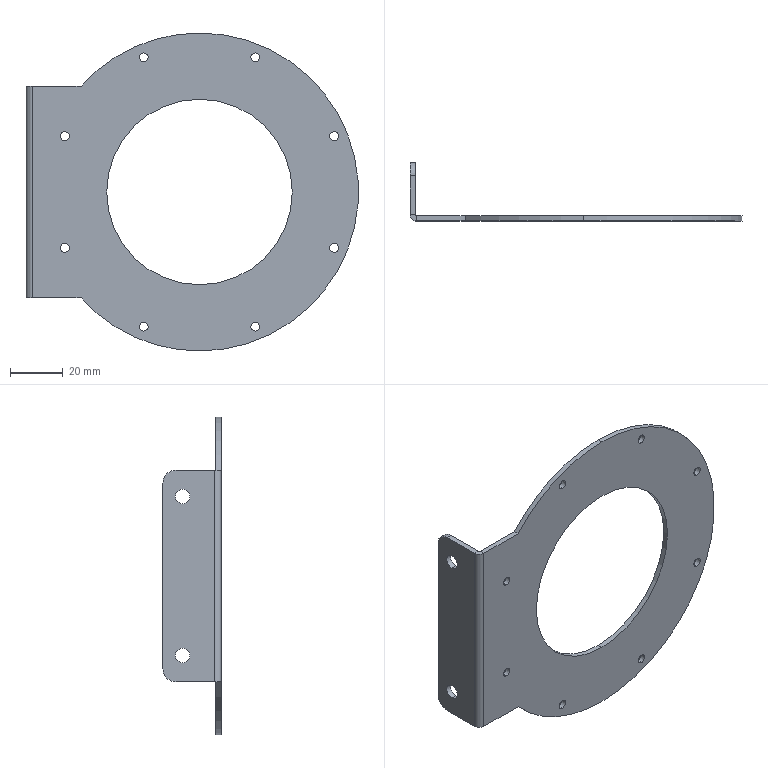Part | SolidWorks | features HoleWzd 2, ICE 2, Fillet 1, FlatPattern 1, SMBaseFlange 1, SheetMetal 1 | 1 solid | 40 faces | box 125.5 x 22 x 120 mm | volume 19406 mm3 | cylinder 29 | plane 11 | commonest cylinder face diameters 3.4 x16 5.5 x4 120 x3 10 x2 70 x2 1 x1
STEP:
#1=CARTESIAN_POINT('',(-2.,12.5,32.75));
#2=VERTEX_POINT('',#1);
#3=CARTESIAN_POINT('',(-2.,12.5,27.25));
#4=VERTEX_POINT('',#3);
#5=CARTESIAN_POINT('',(-2.,12.5,30.));
#6=DIRECTION('',(1.,0.,0.));
#7=DIRECTION('',(0.,0.,-1.));
#8=AXIS2_PLACEMENT_3D('',#5,#6,#7);
#9=CIRCLE('',#8,2.75);
#10=EDGE_CURVE('',#2,#4,#9,.T.);
#11=ORIENTED_EDGE('',*,*,#10,.F.);
#12=CARTESIAN_POINT('',(0.,12.5,32.75));
#13=VERTEX_POINT('',#12);
#14=CARTESIAN_POINT('',(0.,12.5,32.75));
#15=DIRECTION('',(1.,0.,0.));
#16=VECTOR('',#15,1000.);
#17=LINE('',#14,#16);
#18=EDGE_CURVE('',#2,#13,#17,.T.);
#19=ORIENTED_EDGE('',*,*,#18,.T.);
#20=CARTESIAN_POINT('',(0.,12.5,27.25));
#21=VERTEX_POINT('',#20);
#22=CARTESIAN_POINT('',(0.,12.5,30.));
#23=DIRECTION('',(1.,0.,0.));
#24=DIRECTION('',(0.,0.,-1.));
#25=AXIS2_PLACEMENT_3D('',#22,#23,#24);
#26=CIRCLE('',#25,2.75);
#27=EDGE_CURVE('',#13,#21,#26,.T.);
#28=ORIENTED_EDGE('',*,*,#27,.T.);
#29=CARTESIAN_POINT('',(0.,12.5,27.25));
#30=DIRECTION('',(1.,0.,0.));
#31=VECTOR('',#30,1000.);
#32=LINE('',#29,#31);
#33=EDGE_CURVE('',#4,#21,#32,.T.);
#34=ORIENTED_EDGE('',*,*,#33,.F.);
#35=EDGE_LOOP('',(#11,#19,#28,#34));
#36=FACE_OUTER_BOUND('',#35,.T.);
#37=CARTESIAN_POINT('',(0.,12.5,30.));
#38=DIRECTION('',(1.,0.,0.));
#39=DIRECTION('',(0.,0.,-1.));
#40=AXIS2_PLACEMENT_3D('',#37,#38,#39);
#41=CYLINDRICAL_SURFACE('',#40,2.75);
#42=ADVANCED_FACE('',(#36),#41,.F.);
#43=CARTESIAN_POINT('',(-2.,12.5,-27.25));
#44=VERTEX_POINT('',#43);
#45=CARTESIAN_POINT('',(-2.,12.5,-32.75));
#46=VERTEX_POINT('',#45);
#47=CARTESIAN_POINT('',(-2.,12.5,-30.));
#48=DIRECTION('',(1.,0.,0.));
#49=DIRECTION('',(0.,0.,-1.));
#50=AXIS2_PLACEMENT_3D('',#47,#48,#49);
#51=CIRCLE('',#50,2.75);
#52=EDGE_CURVE('',#44,#46,#51,.T.);
#53=ORIENTED_EDGE('',*,*,#52,.F.);
#54=CARTESIAN_POINT('',(0.,12.5,-27.25));
#55=VERTEX_POINT('',#54);
#56=CARTESIAN_POINT('',(0.,12.5,-27.25));
#57=DIRECTION('',(1.,0.,0.));
#58=VECTOR('',#57,1000.);
#59=LINE('',#56,#58);
#60=EDGE_CURVE('',#44,#55,#59,.T.);
#61=ORIENTED_EDGE('',*,*,#60,.T.);
#62=CARTESIAN_POINT('',(0.,12.5,-32.75));
#63=VERTEX_POINT('',#62);
#64=CARTESIAN_POINT('',(0.,12.5,-30.));
#65=DIRECTION('',(1.,0.,0.));
#66=DIRECTION('',(0.,0.,-1.));
#67=AXIS2_PLACEMENT_3D('',#64,#65,#66);
#68=CIRCLE('',#67,2.75);
#69=EDGE_CURVE('',#55,#63,#68,.T.);
#70=ORIENTED_EDGE('',*,*,#69,.T.);
#71=CARTESIAN_POINT('',(0.,12.5,-32.75));
#72=DIRECTION('',(1.,0.,0.));
#73=VECTOR('',#72,1000.);
#74=LINE('',#71,#73);
#75=EDGE_CURVE('',#46,#63,#74,.T.);
#76=ORIENTED_EDGE('',*,*,#75,.F.);
#77=EDGE_LOOP('',(#53,#61,#70,#76));
#78=FACE_OUTER_BOUND('',#77,.T.);
#79=CARTESIAN_POINT('',(0.,12.5,-30.));
#80=DIRECTION('',(1.,0.,0.));
#81=DIRECTION('',(0.,0.,-1.));
#82=AXIS2_PLACEMENT_3D('',#79,#80,#81);
#83=CYLINDRICAL_SURFACE('',#82,2.75);
#84=ADVANCED_FACE('',(#78),#83,.F.);
#85=CARTESIAN_POINT('',(42.452,-2.,-52.513));
#86=VERTEX_POINT('',#85);
#87=CARTESIAN_POINT('',(42.452,-2.,-49.113));
#88=VERTEX_POINT('',#87);
#89=CARTESIAN_POINT('',(42.452,-2.,-50.813));
#90=DIRECTION('',(0.,1.,0.));
#91=DIRECTION('',(0.,0.,1.));
#92=AXIS2_PLACEMENT_3D('',#89,#90,#91);
#93=CIRCLE('',#92,1.7);
#94=EDGE_CURVE('',#86,#88,#93,.T.);
#95=ORIENTED_EDGE('',*,*,#94,.F.);
#96=CARTESIAN_POINT('',(42.452,0.,-52.513));
#97=VERTEX_POINT('',#96);
#98=CARTESIAN_POINT('',(42.452,0.,-52.513));
#99=DIRECTION('',(0.,1.,0.));
#100=VECTOR('',#99,1000.);
#101=LINE('',#98,#100);
#102=EDGE_CURVE('',#86,#97,#101,.T.);
#103=ORIENTED_EDGE('',*,*,#102,.T.);
#104=CARTESIAN_POINT('',(42.452,0.,-49.113));
#105=VERTEX_POINT('',#104);
#106=CARTESIAN_POINT('',(42.452,0.,-50.813));
#107=DIRECTION('',(0.,1.,0.));
#108=DIRECTION('',(0.,0.,1.));
#109=AXIS2_PLACEMENT_3D('',#106,#107,#108);
#110=CIRCLE('',#109,1.7);
#111=EDGE_CURVE('',#97,#105,#110,.T.);
#112=ORIENTED_EDGE('',*,*,#111,.T.);
#113=CARTESIAN_POINT('',(42.452,0.,-49.113));
#114=DIRECTION('',(0.,1.,0.));
#115=VECTOR('',#114,1000.);
#116=LINE('',#113,#115);
#117=EDGE_CURVE('',#88,#105,#116,.T.);
#118=ORIENTED_EDGE('',*,*,#117,.F.);
#119=EDGE_LOOP('',(#95,#103,#112,#118));
#120=FACE_OUTER_BOUND('',#119,.T.);
#121=CARTESIAN_POINT('',(42.452,0.,-50.813));
#122=DIRECTION('',(0.,1.,0.));
#123=DIRECTION('',(0.,0.,1.));
#124=AXIS2_PLACEMENT_3D('',#121,#122,#123);
#125=CYLINDRICAL_SURFACE('',#124,1.7);
#126=ADVANCED_FACE('',(#120),#125,.F.);
#127=CARTESIAN_POINT('',(84.548,-2.,-52.513));
#128=VERTEX_POINT('',#127);
#129=CARTESIAN_POINT('',(84.548,-2.,-49.113));
#130=VERTEX_POINT('',#129);
#131=CARTESIAN_POINT('',(84.548,-2.,-50.813));
#132=DIRECTION('',(0.,1.,0.));
#133=DIRECTION('',(0.,0.,1.));
#134=AXIS2_PLACEMENT_3D('',#131,#132,#133);
#135=CIRCLE('',#134,1.7);
#136=EDGE_CURVE('',#128,#130,#135,.T.);
#137=ORIENTED_EDGE('',*,*,#136,.F.);
#138=CARTESIAN_POINT('',(84.548,0.,-52.513));
#139=VERTEX_POINT('',#138);
#140=CARTESIAN_POINT('',(84.548,0.,-52.513));
#141=DIRECTION('',(0.,1.,0.));
#142=VECTOR('',#141,1000.);
#143=LINE('',#140,#142);
#144=EDGE_CURVE('',#128,#139,#143,.T.);
#145=ORIENTED_EDGE('',*,*,#144,.T.);
#146=CARTESIAN_POINT('',(84.548,0.,-49.113));
#147=VERTEX_POINT('',#146);
#148=CARTESIAN_POINT('',(84.548,0.,-50.813));
#149=DIRECTION('',(0.,1.,0.));
#150=DIRECTION('',(0.,0.,1.));
#151=AXIS2_PLACEMENT_3D('',#148,#149,#150);
#152=CIRCLE('',#151,1.7);
#153=EDGE_CURVE('',#139,#147,#152,.T.);
#154=ORIENTED_EDGE('',*,*,#153,.T.);
#155=CARTESIAN_POINT('',(84.548,0.,-49.113));
#156=DIRECTION('',(0.,1.,0.));
#157=VECTOR('',#156,1000.);
#158=LINE('',#155,#157);
#159=EDGE_CURVE('',#130,#147,#158,.T.);
#160=ORIENTED_EDGE('',*,*,#159,.F.);
#161=EDGE_LOOP('',(#137,#145,#154,#160));
#162=FACE_OUTER_BOUND('',#161,.T.);
#163=CARTESIAN_POINT('',(84.548,0.,-50.813));
#164=DIRECTION('',(0.,1.,0.));
#165=DIRECTION('',(0.,0.,1.));
#166=AXIS2_PLACEMENT_3D('',#163,#164,#165);
#167=CYLINDRICAL_SURFACE('',#166,1.7);
#168=ADVANCED_FACE('',(#162),#167,.F.);
#169=CARTESIAN_POINT('',(114.313,-2.,-22.748));
#170=VERTEX_POINT('',#169);
#171=CARTESIAN_POINT('',(114.313,-2.,-19.348));
#172=VERTEX_POINT('',#171);
#173=CARTESIAN_POINT('',(114.313,-2.,-21.048));
#174=DIRECTION('',(0.,1.,0.));
#175=DIRECTION('',(0.,0.,1.));
#176=AXIS2_PLACEMENT_3D('',#173,#174,#175);
#177=CIRCLE('',#176,1.7);
#178=EDGE_CURVE('',#170,#172,#177,.T.);
#179=ORIENTED_EDGE('',*,*,#178,.F.);
#180=CARTESIAN_POINT('',(114.313,0.,-22.748));
#181=VERTEX_POINT('',#180);
#182=CARTESIAN_POINT('',(114.313,0.,-22.748));
#183=DIRECTION('',(0.,1.,0.));
#184=VECTOR('',#183,1000.);
#185=LINE('',#182,#184);
#186=EDGE_CURVE('',#170,#181,#185,.T.);
#187=ORIENTED_EDGE('',*,*,#186,.T.);
#188=CARTESIAN_POINT('',(114.313,0.,-19.348));
#189=VERTEX_POINT('',#188);
#190=CARTESIAN_POINT('',(114.313,0.,-21.048));
#191=DIRECTION('',(0.,1.,0.));
#192=DIRECTION('',(0.,0.,1.));
#193=AXIS2_PLACEMENT_3D('',#190,#191,#192);
#194=CIRCLE('',#193,1.7);
#195=EDGE_CURVE('',#181,#189,#194,.T.);
#196=ORIENTED_EDGE('',*,*,#195,.T.);
#197=CARTESIAN_POINT('',(114.313,0.,-19.348));
#198=DIRECTION('',(0.,1.,0.));
#199=VECTOR('',#198,1000.);
#200=LINE('',#197,#199);
#201=EDGE_CURVE('',#172,#189,#200,.T.);
#202=ORIENTED_EDGE('',*,*,#201,.F.);
#203=EDGE_LOOP('',(#179,#187,#196,#202));
#204=FACE_OUTER_BOUND('',#203,.T.);
#205=CARTESIAN_POINT('',(114.313,0.,-21.048));
#206=DIRECTION('',(0.,1.,0.));
#207=DIRECTION('',(0.,0.,1.));
#208=AXIS2_PLACEMENT_3D('',#205,#206,#207);
#209=CYLINDRICAL_SURFACE('',#208,1.7);
#210=ADVANCED_FACE('',(#204),#209,.F.);
#211=CARTESIAN_POINT('',(114.313,-2.,19.348));
#212=VERTEX_POINT('',#211);
#213=CARTESIAN_POINT('',(114.313,-2.,22.748));
#214=VERTEX_POINT('',#213);
#215=CARTESIAN_POINT('',(114.313,-2.,21.048));
#216=DIRECTION('',(0.,1.,0.));
#217=DIRECTION('',(0.,0.,1.));
#218=AXIS2_PLACEMENT_3D('',#215,#216,#217);
#219=CIRCLE('',#218,1.7);
#220=EDGE_CURVE('',#212,#214,#219,.T.);
#221=ORIENTED_EDGE('',*,*,#220,.F.);
#222=CARTESIAN_POINT('',(114.313,0.,19.348));
#223=VERTEX_POINT('',#222);
#224=CARTESIAN_POINT('',(114.313,0.,19.348));
#225=DIRECTION('',(0.,1.,0.));
#226=VECTOR('',#225,1000.);
#227=LINE('',#224,#226);
#228=EDGE_CURVE('',#212,#223,#227,.T.);
#229=ORIENTED_EDGE('',*,*,#228,.T.);
#230=CARTESIAN_POINT('',(114.313,0.,22.748));
#231=VERTEX_POINT('',#230);
#232=CARTESIAN_POINT('',(114.313,0.,21.048));
#233=DIRECTION('',(0.,1.,0.));
#234=DIRECTION('',(0.,0.,1.));
#235=AXIS2_PLACEMENT_3D('',#232,#233,#234);
#236=CIRCLE('',#235,1.7);
#237=EDGE_CURVE('',#223,#231,#236,.T.);
#238=ORIENTED_EDGE('',*,*,#237,.T.);
#239=CARTESIAN_POINT('',(114.313,0.,22.748));
#240=DIRECTION('',(0.,1.,0.));
#241=VECTOR('',#240,1000.);
#242=LINE('',#239,#241);
#243=EDGE_CURVE('',#214,#231,#242,.T.);
#244=ORIENTED_EDGE('',*,*,#243,.F.);
#245=EDGE_LOOP('',(#221,#229,#238,#244));
#246=FACE_OUTER_BOUND('',#245,.T.);
#247=CARTESIAN_POINT('',(114.313,0.,21.048));
#248=DIRECTION('',(0.,1.,0.));
#249=DIRECTION('',(0.,0.,1.));
#250=AXIS2_PLACEMENT_3D('',#247,#248,#249);
#251=CYLINDRICAL_SURFACE('',#250,1.7);
#252=ADVANCED_FACE('',(#246),#251,.F.);
#253=CARTESIAN_POINT('',(84.548,-2.,49.113));
#254=VERTEX_POINT('',#253);
#255=CARTESIAN_POINT('',(84.548,-2.,52.513));
#256=VERTEX_POINT('',#255);
#257=CARTESIAN_POINT('',(84.548,-2.,50.813));
#258=DIRECTION('',(0.,1.,0.));
#259=DIRECTION('',(0.,0.,1.));
#260=AXIS2_PLACEMENT_3D('',#257,#258,#259);
#261=CIRCLE('',#260,1.7);
#262=EDGE_CURVE('',#254,#256,#261,.T.);
#263=ORIENTED_EDGE('',*,*,#262,.F.);
#264=CARTESIAN_POINT('',(84.548,0.,49.113));
#265=VERTEX_POINT('',#264);
#266=CARTESIAN_POINT('',(84.548,0.,49.113));
#267=DIRECTION('',(0.,1.,0.));
#268=VECTOR('',#267,1000.);
#269=LINE('',#266,#268);
#270=EDGE_CURVE('',#254,#265,#269,.T.);
#271=ORIENTED_EDGE('',*,*,#270,.T.);
#272=CARTESIAN_POINT('',(84.548,0.,52.513));
#273=VERTEX_POINT('',#272);
#274=CARTESIAN_POINT('',(84.548,0.,50.813));
#275=DIRECTION('',(0.,1.,0.));
#276=DIRECTION('',(0.,0.,1.));
#277=AXIS2_PLACEMENT_3D('',#274,#275,#276);
#278=CIRCLE('',#277,1.7);
#279=EDGE_CURVE('',#265,#273,#278,.T.);
#280=ORIENTED_EDGE('',*,*,#279,.T.);
#281=CARTESIAN_POINT('',(84.548,0.,52.513));
#282=DIRECTION('',(0.,1.,0.));
#283=VECTOR('',#282,1000.);
#284=LINE('',#281,#283);
#285=EDGE_CURVE('',#256,#273,#284,.T.);
#286=ORIENTED_EDGE('',*,*,#285,.F.);
#287=EDGE_LOOP('',(#263,#271,#280,#286));
#288=FACE_OUTER_BOUND('',#287,.T.);
#289=CARTESIAN_POINT('',(84.548,0.,50.813));
#290=DIRECTION('',(0.,1.,0.));
#291=DIRECTION('',(0.,0.,1.));
#292=AXIS2_PLACEMENT_3D('',#289,#290,#291);
#293=CYLINDRICAL_SURFACE('',#292,1.7);
#294=ADVANCED_FACE('',(#288),#293,.F.);
#295=CARTESIAN_POINT('',(42.452,-2.,49.113));
#296=VERTEX_POINT('',#295);
#297=CARTESIAN_POINT('',(42.452,-2.,52.513));
#298=VERTEX_POINT('',#297);
#299=CARTESIAN_POINT('',(42.452,-2.,50.813));
#300=DIRECTION('',(0.,1.,0.));
#301=DIRECTION('',(0.,0.,1.));
#302=AXIS2_PLACEMENT_3D('',#299,#300,#301);
#303=CIRCLE('',#302,1.7);
#304=EDGE_CURVE('',#296,#298,#303,.T.);
#305=ORIENTED_EDGE('',*,*,#304,.F.);
#306=CARTESIAN_POINT('',(42.452,0.,49.113));
#307=VERTEX_POINT('',#306);
#308=CARTESIAN_POINT('',(42.452,0.,49.113));
#309=DIRECTION('',(0.,1.,0.));
#310=VECTOR('',#309,1000.);
#311=LINE('',#308,#310);
#312=EDGE_CURVE('',#296,#307,#311,.T.);
#313=ORIENTED_EDGE('',*,*,#312,.T.);
#314=CARTESIAN_POINT('',(42.452,0.,52.513));
#315=VERTEX_POINT('',#314);
#316=CARTESIAN_POINT('',(42.452,0.,50.813));
#317=DIRECTION('',(0.,1.,0.));
#318=DIRECTION('',(0.,0.,1.));
#319=AXIS2_PLACEMENT_3D('',#316,#317,#318);
#320=CIRCLE('',#319,1.7);
#321=EDGE_CURVE('',#307,#315,#320,.T.);
#322=ORIENTED_EDGE('',*,*,#321,.T.);
#323=CARTESIAN_POINT('',(42.452,0.,52.513));
#324=DIRECTION('',(0.,1.,0.));
#325=VECTOR('',#324,1000.);
#326=LINE('',#323,#325);
#327=EDGE_CURVE('',#298,#315,#326,.T.);
#328=ORIENTED_EDGE('',*,*,#327,.F.);
#329=EDGE_LOOP('',(#305,#313,#322,#328));
#330=FACE_OUTER_BOUND('',#329,.T.);
#331=CARTESIAN_POINT('',(42.452,0.,50.813));
#332=DIRECTION('',(0.,1.,0.));
#333=DIRECTION('',(0.,0.,1.));
#334=AXIS2_PLACEMENT_3D('',#331,#332,#333);
#335=CYLINDRICAL_SURFACE('',#334,1.7);
#336=ADVANCED_FACE('',(#330),#335,.F.);
#337=CARTESIAN_POINT('',(12.687,-2.,19.348));
#338=VERTEX_POINT('',#337);
#339=CARTESIAN_POINT('',(12.687,-2.,22.748));
#340=VERTEX_POINT('',#339);
#341=CARTESIAN_POINT('',(12.687,-2.,21.048));
#342=DIRECTION('',(0.,1.,0.));
#343=DIRECTION('',(0.,0.,1.));
#344=AXIS2_PLACEMENT_3D('',#341,#342,#343);
#345=CIRCLE('',#344,1.7);
#346=EDGE_CURVE('',#338,#340,#345,.T.);
#347=ORIENTED_EDGE('',*,*,#346,.F.);
#348=CARTESIAN_POINT('',(12.687,0.,19.348));
#349=VERTEX_POINT('',#348);
#350=CARTESIAN_POINT('',(12.687,0.,19.348));
#351=DIRECTION('',(0.,1.,0.));
#352=VECTOR('',#351,1000.);
#353=LINE('',#350,#352);
#354=EDGE_CURVE('',#338,#349,#353,.T.);
#355=ORIENTED_EDGE('',*,*,#354,.T.);
#356=CARTESIAN_POINT('',(12.687,0.,22.748));
#357=VERTEX_POINT('',#356);
#358=CARTESIAN_POINT('',(12.687,0.,21.048));
#359=DIRECTION('',(0.,1.,0.));
#360=DIRECTION('',(0.,0.,1.));
#361=AXIS2_PLACEMENT_3D('',#358,#359,#360);
#362=CIRCLE('',#361,1.7);
#363=EDGE_CURVE('',#349,#357,#362,.T.);
#364=ORIENTED_EDGE('',*,*,#363,.T.);
#365=CARTESIAN_POINT('',(12.687,0.,22.748));
#366=DIRECTION('',(0.,1.,0.));
#367=VECTOR('',#366,1000.);
#368=LINE('',#365,#367);
#369=EDGE_CURVE('',#340,#357,#368,.T.);
#370=ORIENTED_EDGE('',*,*,#369,.F.);
#371=EDGE_LOOP('',(#347,#355,#364,#370));
#372=FACE_OUTER_BOUND('',#371,.T.);
#373=CARTESIAN_POINT('',(12.687,0.,21.048));
#374=DIRECTION('',(0.,1.,0.));
#375=DIRECTION('',(0.,0.,1.));
#376=AXIS2_PLACEMENT_3D('',#373,#374,#375);
#377=CYLINDRICAL_SURFACE('',#376,1.7);
#378=ADVANCED_FACE('',(#372),#377,.F.);
#379=CARTESIAN_POINT('',(12.687,-2.,-22.748));
#380=VERTEX_POINT('',#379);
#381=CARTESIAN_POINT('',(12.687,-2.,-19.348));
#382=VERTEX_POINT('',#381);
#383=CARTESIAN_POINT('',(12.687,-2.,-21.048));
#384=DIRECTION('',(0.,1.,0.));
#385=DIRECTION('',(0.,0.,1.));
#386=AXIS2_PLACEMENT_3D('',#383,#384,#385);
#387=CIRCLE('',#386,1.7);
#388=EDGE_CURVE('',#380,#382,#387,.T.);
#389=ORIENTED_EDGE('',*,*,#388,.F.);
#390=CARTESIAN_POINT('',(12.687,0.,-22.748));
#391=VERTEX_POINT('',#390);
#392=CARTESIAN_POINT('',(12.687,0.,-22.748));
#393=DIRECTION('',(0.,1.,0.));
#394=VECTOR('',#393,1000.);
#395=LINE('',#392,#394);
#396=EDGE_CURVE('',#380,#391,#395,.T.);
#397=ORIENTED_EDGE('',*,*,#396,.T.);
#398=CARTESIAN_POINT('',(12.687,0.,-19.348));
#399=VERTEX_POINT('',#398);
#400=CARTESIAN_POINT('',(12.687,0.,-21.048));
#401=DIRECTION('',(0.,1.,0.));
#402=DIRECTION('',(0.,0.,1.));
#403=AXIS2_PLACEMENT_3D('',#400,#401,#402);
#404=CIRCLE('',#403,1.7);
#405=EDGE_CURVE('',#391,#399,#404,.T.);
#406=ORIENTED_EDGE('',*,*,#405,.T.);
#407=CARTESIAN_POINT('',(12.687,0.,-19.348));
#408=DIRECTION('',(0.,1.,0.));
#409=VECTOR('',#408,1000.);
#410=LINE('',#407,#409);
#411=EDGE_CURVE('',#382,#399,#410,.T.);
#412=ORIENTED_EDGE('',*,*,#411,.F.);
#413=EDGE_LOOP('',(#389,#397,#406,#412));
#414=FACE_OUTER_BOUND('',#413,.T.);
#415=CARTESIAN_POINT('',(12.687,0.,-21.048));
#416=DIRECTION('',(0.,1.,0.));
#417=DIRECTION('',(0.,0.,1.));
#418=AXIS2_PLACEMENT_3D('',#415,#416,#417);
#419=CYLINDRICAL_SURFACE('',#418,1.7);
#420=ADVANCED_FACE('',(#414),#419,.F.);
#421=CARTESIAN_POINT('',(63.5,-2.,35.));
#422=VERTEX_POINT('',#421);
#423=CARTESIAN_POINT('',(63.5,-2.,-35.));
#424=VERTEX_POINT('',#423);
#425=CARTESIAN_POINT('',(63.5,-2.,0.));
#426=DIRECTION('',(0.,-1.,0.));
#427=DIRECTION('',(0.,0.,1.));
#428=AXIS2_PLACEMENT_3D('',#425,#426,#427);
#429=CIRCLE('',#428,35.);
#430=EDGE_CURVE('',#422,#424,#429,.T.);
#431=ORIENTED_EDGE('',*,*,#430,.T.);
#432=CARTESIAN_POINT('',(63.5,0.,-35.));
#433=VERTEX_POINT('',#432);
#434=CARTESIAN_POINT('',(63.5,-100.995,-35.));
#435=DIRECTION('',(0.,1.,0.));
#436=VECTOR('',#435,1000.);
#437=LINE('',#434,#436);
#438=EDGE_CURVE('',#424,#433,#437,.T.);
#439=ORIENTED_EDGE('',*,*,#438,.T.);
#440=CARTESIAN_POINT('',(63.5,0.,35.));
#441=VERTEX_POINT('',#440);
#442=CARTESIAN_POINT('',(63.5,0.,0.));
#443=DIRECTION('',(0.,1.,0.));
#444=DIRECTION('',(0.,0.,1.));
#445=AXIS2_PLACEMENT_3D('',#442,#443,#444);
#446=CIRCLE('',#445,35.);
#447=EDGE_CURVE('',#433,#441,#446,.T.);
#448=ORIENTED_EDGE('',*,*,#447,.T.);
#449=CARTESIAN_POINT('',(63.5,-100.995,35.));
#450=DIRECTION('',(0.,1.,0.));
#451=VECTOR('',#450,1000.);
#452=LINE('',#449,#451);
#453=EDGE_CURVE('',#422,#441,#452,.T.);
#454=ORIENTED_EDGE('',*,*,#453,.F.);
#455=EDGE_LOOP('',(#431,#439,#448,#454));
#456=FACE_OUTER_BOUND('',#455,.T.);
#457=CARTESIAN_POINT('',(63.5,-100.995,0.));
#458=DIRECTION('',(0.,1.,0.));
#459=DIRECTION('',(0.,0.,1.));
#460=AXIS2_PLACEMENT_3D('',#457,#458,#459);
#461=CYLINDRICAL_SURFACE('',#460,35.);
#462=ADVANCED_FACE('',(#456),#461,.F.);
#463=CARTESIAN_POINT('',(63.5,-2.,-60.));
#464=VERTEX_POINT('',#463);
#465=CARTESIAN_POINT('',(63.5,-2.,60.));
#466=VERTEX_POINT('',#465);
#467=CARTESIAN_POINT('',(63.5,-2.,0.));
#468=DIRECTION('',(0.,-1.,0.));
#469=DIRECTION('',(0.,0.,1.));
#470=AXIS2_PLACEMENT_3D('',#467,#468,#469);
#471=CIRCLE('',#470,60.);
#472=EDGE_CURVE('',#464,#466,#471,.T.);
#473=ORIENTED_EDGE('',*,*,#472,.F.);
#474=CARTESIAN_POINT('',(63.5,0.,-60.));
#475=VERTEX_POINT('',#474);
#476=CARTESIAN_POINT('',(63.5,-171.706,-60.));
#477=DIRECTION('',(0.,1.,0.));
#478=VECTOR('',#477,1000.);
#479=LINE('',#476,#478);
#480=EDGE_CURVE('',#464,#475,#479,.T.);
#481=ORIENTED_EDGE('',*,*,#480,.T.);
#482=CARTESIAN_POINT('',(63.5,0.,60.));
#483=VERTEX_POINT('',#482);
#484=CARTESIAN_POINT('',(63.5,0.,0.));
#485=DIRECTION('',(0.,1.,0.));
#486=DIRECTION('',(0.,0.,1.));
#487=AXIS2_PLACEMENT_3D('',#484,#485,#486);
#488=CIRCLE('',#487,60.);
#489=EDGE_CURVE('',#483,#475,#488,.T.);
#490=ORIENTED_EDGE('',*,*,#489,.F.);
#491=CARTESIAN_POINT('',(63.5,-171.706,60.));
#492=DIRECTION('',(0.,1.,0.));
#493=VECTOR('',#492,1000.);
#494=LINE('',#491,#493);
#495=EDGE_CURVE('',#466,#483,#494,.T.);
#496=ORIENTED_EDGE('',*,*,#495,.F.);
#497=EDGE_LOOP('',(#473,#481,#490,#496));
#498=FACE_OUTER_BOUND('',#497,.T.);
#499=CARTESIAN_POINT('',(63.5,-171.706,0.));
#500=DIRECTION('',(0.,1.,0.));
#501=DIRECTION('',(0.,0.,1.));
#502=AXIS2_PLACEMENT_3D('',#499,#500,#501);
#503=CYLINDRICAL_SURFACE('',#502,60.);
#504=ADVANCED_FACE('',(#498),#503,.T.);
#505=CARTESIAN_POINT('',(18.779,-2.,40.));
#506=VERTEX_POINT('',#505);
#507=CARTESIAN_POINT('',(63.5,-2.,0.));
#508=DIRECTION('',(0.,-1.,0.));
#509=DIRECTION('',(0.,0.,1.));
#510=AXIS2_PLACEMENT_3D('',#507,#508,#509);
#511=CIRCLE('',#510,60.);
#512=EDGE_CURVE('',#466,#506,#511,.T.);
#513=ORIENTED_EDGE('',*,*,#512,.F.);
#514=ORIENTED_EDGE('',*,*,#495,.T.);
#515=CARTESIAN_POINT('',(18.779,0.,40.));
#516=VERTEX_POINT('',#515);
#517=CARTESIAN_POINT('',(63.5,0.,0.));
#518=DIRECTION('',(0.,1.,0.));
#519=DIRECTION('',(0.,0.,1.));
#520=AXIS2_PLACEMENT_3D('',#517,#518,#519);
#521=CIRCLE('',#520,60.);
#522=EDGE_CURVE('',#516,#483,#521,.T.);
#523=ORIENTED_EDGE('',*,*,#522,.F.);
#524=CARTESIAN_POINT('',(18.779,-171.706,40.));
#525=DIRECTION('',(0.,-1.,0.));
#526=VECTOR('',#525,1000.);
#527=LINE('',#524,#526);
#528=EDGE_CURVE('',#516,#506,#527,.T.);
#529=ORIENTED_EDGE('',*,*,#528,.T.);
#530=EDGE_LOOP('',(#513,#514,#523,#529));
#531=FACE_OUTER_BOUND('',#530,.T.);
#532=CARTESIAN_POINT('',(63.5,-171.706,0.));
#533=DIRECTION('',(0.,1.,0.));
#534=DIRECTION('',(0.,0.,1.));
#535=AXIS2_PLACEMENT_3D('',#532,#533,#534);
#536=CYLINDRICAL_SURFACE('',#535,60.);
#537=ADVANCED_FACE('',(#531),#536,.T.);
#538=CARTESIAN_POINT('',(0.5,0.,40.));
#539=VERTEX_POINT('',#538);
#540=CARTESIAN_POINT('',(0.5,-2.,40.));
#541=VERTEX_POINT('',#540);
#542=CARTESIAN_POINT('',(0.5,0.,40.));
#543=DIRECTION('',(0.,-1.,0.));
#544=VECTOR('',#543,1000.);
#545=LINE('',#542,#544);
#546=EDGE_CURVE('',#539,#541,#545,.T.);
#547=ORIENTED_EDGE('',*,*,#546,.F.);
#548=CARTESIAN_POINT('',(0.,0.5,40.));
#549=VERTEX_POINT('',#548);
#550=CARTESIAN_POINT('',(0.5,0.5,40.));
#551=DIRECTION('',(0.,0.,1.));
#552=DIRECTION('',(-1.,0.,0.));
#553=AXIS2_PLACEMENT_3D('',#550,#551,#552);
#554=CIRCLE('',#553,0.5);
#555=EDGE_CURVE('',#549,#539,#554,.T.);
#556=ORIENTED_EDGE('',*,*,#555,.F.);
#557=CARTESIAN_POINT('',(-2.,0.5,40.));
#558=VERTEX_POINT('',#557);
#559=CARTESIAN_POINT('',(-2.,0.5,40.));
#560=DIRECTION('',(1.,0.,0.));
#561=VECTOR('',#560,1000.);
#562=LINE('',#559,#561);
#563=EDGE_CURVE('',#558,#549,#562,.T.);
#564=ORIENTED_EDGE('',*,*,#563,.F.);
#565=CARTESIAN_POINT('',(0.5,0.5,40.));
#566=DIRECTION('',(0.,0.,1.));
#567=DIRECTION('',(1.,0.,0.));
#568=AXIS2_PLACEMENT_3D('',#565,#566,#567);
#569=CIRCLE('',#568,2.5);
#570=EDGE_CURVE('',#558,#541,#569,.T.);
#571=ORIENTED_EDGE('',*,*,#570,.T.);
#572=EDGE_LOOP('',(#547,#556,#564,#571));
#573=FACE_OUTER_BOUND('',#572,.T.);
#574=CARTESIAN_POINT('',(0.5,0.,40.));
#575=DIRECTION('',(0.,0.,1.));
#576=DIRECTION('',(1.,0.,0.));
#577=AXIS2_PLACEMENT_3D('',#574,#575,#576);
#578=PLANE('',#577);
#579=ADVANCED_FACE('',(#573),#578,.T.);
#580=ORIENTED_EDGE('',*,*,#528,.F.);
#581=CARTESIAN_POINT('',(0.,0.,40.));
#582=DIRECTION('',(1.,0.,0.));
#583=VECTOR('',#582,1000.);
#584=LINE('',#581,#583);
#585=EDGE_CURVE('',#539,#516,#584,.T.);
#586=ORIENTED_EDGE('',*,*,#585,.F.);
#587=ORIENTED_EDGE('',*,*,#546,.T.);
#588=CARTESIAN_POINT('',(0.,-2.,40.));
#589=DIRECTION('',(1.,0.,0.));
#590=VECTOR('',#589,1000.);
#591=LINE('',#588,#590);
#592=EDGE_CURVE('',#541,#506,#591,.T.);
#593=ORIENTED_EDGE('',*,*,#592,.T.);
#594=EDGE_LOOP('',(#580,#586,#587,#593));
#595=FACE_OUTER_BOUND('',#594,.T.);
#596=CARTESIAN_POINT('',(-2.,0.5,40.));
#597=DIRECTION('',(0.,0.,1.));
#598=DIRECTION('',(1.,0.,0.));
#599=AXIS2_PLACEMENT_3D('',#596,#597,#598);
#600=PLANE('',#599);
#601=ADVANCED_FACE('',(#595),#600,.T.);
#602=CARTESIAN_POINT('',(0.,0.5,-40.));
#603=VERTEX_POINT('',#602);
#604=CARTESIAN_POINT('',(-2.,0.5,-40.));
#605=VERTEX_POINT('',#604);
#606=CARTESIAN_POINT('',(0.,0.5,-40.));
#607=DIRECTION('',(-1.,0.,0.));
#608=VECTOR('',#607,1000.);
#609=LINE('',#606,#608);
#610=EDGE_CURVE('',#603,#605,#609,.T.);
#611=ORIENTED_EDGE('',*,*,#610,.F.);
#612=CARTESIAN_POINT('',(0.5,0.,-40.));
#613=VERTEX_POINT('',#612);
#614=CARTESIAN_POINT('',(0.5,0.5,-40.));
#615=DIRECTION('',(0.,0.,1.));
#616=DIRECTION('',(-1.,0.,0.));
#617=AXIS2_PLACEMENT_3D('',#614,#615,#616);
#618=CIRCLE('',#617,0.5);
#619=EDGE_CURVE('',#603,#613,#618,.T.);
#620=ORIENTED_EDGE('',*,*,#619,.T.);
#621=CARTESIAN_POINT('',(0.5,-2.,-40.));
#622=VERTEX_POINT('',#621);
#623=CARTESIAN_POINT('',(0.5,-2.,-40.));
#624=DIRECTION('',(0.,1.,0.));
#625=VECTOR('',#624,1000.);
#626=LINE('',#623,#625);
#627=EDGE_CURVE('',#622,#613,#626,.T.);
#628=ORIENTED_EDGE('',*,*,#627,.F.);
#629=CARTESIAN_POINT('',(0.5,0.5,-40.));
#630=DIRECTION('',(0.,0.,1.));
#631=DIRECTION('',(1.,0.,0.));
#632=AXIS2_PLACEMENT_3D('',#629,#630,#631);
#633=CIRCLE('',#632,2.5);
#634=EDGE_CURVE('',#605,#622,#633,.T.);
#635=ORIENTED_EDGE('',*,*,#634,.F.);
#636=EDGE_LOOP('',(#611,#620,#628,#635));
#637=FACE_OUTER_BOUND('',#636,.T.);
#638=CARTESIAN_POINT('',(0.,0.5,-40.));
#639=DIRECTION('',(0.,0.,-1.));
#640=DIRECTION('',(-1.,0.,0.));
#641=AXIS2_PLACEMENT_3D('',#638,#639,#640);
#642=PLANE('',#641);
#643=ADVANCED_FACE('',(#637),#642,.T.);
#644=CARTESIAN_POINT('',(-2.,15.,-40.));
#645=VERTEX_POINT('',#644);
#646=CARTESIAN_POINT('',(-2.,20.,-40.));
#647=DIRECTION('',(0.,-1.,0.));
#648=VECTOR('',#647,1000.);
#649=LINE('',#646,#648);
#650=EDGE_CURVE('',#645,#605,#649,.T.);
#651=ORIENTED_EDGE('',*,*,#650,.F.);
#652=CARTESIAN_POINT('',(0.,15.,-40.));
#653=VERTEX_POINT('',#652);
#654=CARTESIAN_POINT('',(0.5,15.,-40.));
#655=DIRECTION('',(1.,0.,0.));
#656=VECTOR('',#655,1000.);
#657=LINE('',#654,#656);
#658=EDGE_CURVE('',#645,#653,#657,.T.);
#659=ORIENTED_EDGE('',*,*,#658,.T.);
#660=CARTESIAN_POINT('',(0.,20.,-40.));
#661=DIRECTION('',(0.,-1.,0.));
#662=VECTOR('',#661,1000.);
#663=LINE('',#660,#662);
#664=EDGE_CURVE('',#653,#603,#663,.T.);
#665=ORIENTED_EDGE('',*,*,#664,.T.);
#666=ORIENTED_EDGE('',*,*,#610,.T.);
#667=EDGE_LOOP('',(#651,#659,#665,#666));
#668=FACE_OUTER_BOUND('',#667,.T.);
#669=CARTESIAN_POINT('',(0.5,-2.,-40.));
#670=DIRECTION('',(0.,0.,-1.));
#671=DIRECTION('',(-1.,0.,0.));
#672=AXIS2_PLACEMENT_3D('',#669,#670,#671);
#673=PLANE('',#672);
#674=ADVANCED_FACE('',(#668),#673,.T.);
#675=CARTESIAN_POINT('',(42.452,-2.,-50.813));
#676=DIRECTION('',(0.,1.,0.));
#677=DIRECTION('',(0.,0.,1.));
#678=AXIS2_PLACEMENT_3D('',#675,#676,#677);
#679=CIRCLE('',#678,1.7);
#680=EDGE_CURVE('',#88,#86,#679,.T.);
#681=ORIENTED_EDGE('',*,*,#680,.T.);
#682=ORIENTED_EDGE('',*,*,#94,.T.);
#683=EDGE_LOOP('',(#681,#682));
#684=FACE_BOUND('',#683,.T.);
#685=CARTESIAN_POINT('',(84.548,-2.,-50.813));
#686=DIRECTION('',(0.,1.,0.));
#687=DIRECTION('',(0.,0.,1.));
#688=AXIS2_PLACEMENT_3D('',#685,#686,#687);
#689=CIRCLE('',#688,1.7);
#690=EDGE_CURVE('',#130,#128,#689,.T.);
#691=ORIENTED_EDGE('',*,*,#690,.T.);
#692=ORIENTED_EDGE('',*,*,#136,.T.);
#693=EDGE_LOOP('',(#691,#692));
#694=FACE_BOUND('',#693,.T.);
#695=CARTESIAN_POINT('',(114.313,-2.,-21.048));
#696=DIRECTION('',(0.,1.,0.));
#697=DIRECTION('',(0.,0.,1.));
#698=AXIS2_PLACEMENT_3D('',#695,#696,#697);
#699=CIRCLE('',#698,1.7);
#700=EDGE_CURVE('',#172,#170,#699,.T.);
#701=ORIENTED_EDGE('',*,*,#700,.T.);
#702=ORIENTED_EDGE('',*,*,#178,.T.);
#703=EDGE_LOOP('',(#701,#702));
#704=FACE_BOUND('',#703,.T.);
#705=CARTESIAN_POINT('',(114.313,-2.,21.048));
#706=DIRECTION('',(0.,1.,0.));
#707=DIRECTION('',(0.,0.,1.));
#708=AXIS2_PLACEMENT_3D('',#705,#706,#707);
#709=CIRCLE('',#708,1.7);
#710=EDGE_CURVE('',#214,#212,#709,.T.);
#711=ORIENTED_EDGE('',*,*,#710,.T.);
#712=ORIENTED_EDGE('',*,*,#220,.T.);
#713=EDGE_LOOP('',(#711,#712));
#714=FACE_BOUND('',#713,.T.);
#715=CARTESIAN_POINT('',(84.548,-2.,50.813));
#716=DIRECTION('',(0.,1.,0.));
#717=DIRECTION('',(0.,0.,1.));
#718=AXIS2_PLACEMENT_3D('',#715,#716,#717);
#719=CIRCLE('',#718,1.7);
#720=EDGE_CURVE('',#256,#254,#719,.T.);
#721=ORIENTED_EDGE('',*,*,#720,.T.);
#722=ORIENTED_EDGE('',*,*,#262,.T.);
#723=EDGE_LOOP('',(#721,#722));
#724=FACE_BOUND('',#723,.T.);
#725=CARTESIAN_POINT('',(42.452,-2.,50.813));
#726=DIRECTION('',(0.,1.,0.));
#727=DIRECTION('',(0.,0.,1.));
#728=AXIS2_PLACEMENT_3D('',#725,#726,#727);
#729=CIRCLE('',#728,1.7);
#730=EDGE_CURVE('',#298,#296,#729,.T.);
#731=ORIENTED_EDGE('',*,*,#730,.T.);
#732=ORIENTED_EDGE('',*,*,#304,.T.);
#733=EDGE_LOOP('',(#731,#732));
#734=FACE_BOUND('',#733,.T.);
#735=CARTESIAN_POINT('',(12.687,-2.,21.048));
#736=DIRECTION('',(0.,1.,0.));
#737=DIRECTION('',(0.,0.,1.));
#738=AXIS2_PLACEMENT_3D('',#735,#736,#737);
#739=CIRCLE('',#738,1.7);
#740=EDGE_CURVE('',#340,#338,#739,.T.);
#741=ORIENTED_EDGE('',*,*,#740,.T.);
#742=ORIENTED_EDGE('',*,*,#346,.T.);
#743=EDGE_LOOP('',(#741,#742));
#744=FACE_BOUND('',#743,.T.);
#745=CARTESIAN_POINT('',(12.687,-2.,-21.048));
#746=DIRECTION('',(0.,1.,0.));
#747=DIRECTION('',(0.,0.,1.));
#748=AXIS2_PLACEMENT_3D('',#745,#746,#747);
#749=CIRCLE('',#748,1.7);
#750=EDGE_CURVE('',#382,#380,#749,.T.);
#751=ORIENTED_EDGE('',*,*,#750,.T.);
#752=ORIENTED_EDGE('',*,*,#388,.T.);
#753=EDGE_LOOP('',(#751,#752));
#754=FACE_BOUND('',#753,.T.);
#755=ORIENTED_EDGE('',*,*,#430,.F.);
#756=CARTESIAN_POINT('',(63.5,-2.,0.));
#757=DIRECTION('',(0.,-1.,0.));
#758=DIRECTION('',(0.,0.,1.));
#759=AXIS2_PLACEMENT_3D('',#756,#757,#758);
#760=CIRCLE('',#759,35.);
#761=EDGE_CURVE('',#424,#422,#760,.T.);
#762=ORIENTED_EDGE('',*,*,#761,.F.);
#763=EDGE_LOOP('',(#755,#762));
#764=FACE_BOUND('',#763,.T.);
#765=CARTESIAN_POINT('',(18.779,-2.,-40.));
#766=VERTEX_POINT('',#765);
#767=CARTESIAN_POINT('',(63.5,-2.,0.));
#768=DIRECTION('',(0.,-1.,0.));
#769=DIRECTION('',(0.,0.,1.));
#770=AXIS2_PLACEMENT_3D('',#767,#768,#769);
#771=CIRCLE('',#770,60.);
#772=EDGE_CURVE('',#766,#464,#771,.T.);
#773=ORIENTED_EDGE('',*,*,#772,.T.);
#774=ORIENTED_EDGE('',*,*,#472,.T.);
#775=ORIENTED_EDGE('',*,*,#512,.T.);
#776=ORIENTED_EDGE('',*,*,#592,.F.);
#777=CARTESIAN_POINT('',(0.5,-2.,40.));
#778=DIRECTION('',(0.,0.,-1.));
#779=VECTOR('',#778,1000.);
#780=LINE('',#777,#779);
#781=EDGE_CURVE('',#541,#622,#780,.T.);
#782=ORIENTED_EDGE('',*,*,#781,.T.);
#783=CARTESIAN_POINT('',(0.,-2.,-40.));
#784=DIRECTION('',(1.,0.,0.));
#785=VECTOR('',#784,1000.);
#786=LINE('',#783,#785);
#787=EDGE_CURVE('',#622,#766,#786,.T.);
#788=ORIENTED_EDGE('',*,*,#787,.T.);
#789=EDGE_LOOP('',(#773,#774,#775,#776,#782,#788));
#790=FACE_OUTER_BOUND('',#789,.T.);
#791=CARTESIAN_POINT('',(0.,-2.,40.));
#792=DIRECTION('',(0.,1.,0.));
#793=DIRECTION('',(0.,0.,1.));
#794=AXIS2_PLACEMENT_3D('',#791,#792,#793);
#795=PLANE('',#794);
#796=ADVANCED_FACE('',(#684,#694,#704,#714,#724,#734,#744,#754,#764,#790),#795,.F.);
#797=CARTESIAN_POINT('',(42.452,0.,-50.813));
#798=DIRECTION('',(0.,1.,0.));
#799=DIRECTION('',(0.,0.,1.));
#800=AXIS2_PLACEMENT_3D('',#797,#798,#799);
#801=CIRCLE('',#800,1.7);
#802=EDGE_CURVE('',#105,#97,#801,.T.);
#803=ORIENTED_EDGE('',*,*,#802,.F.);
#804=ORIENTED_EDGE('',*,*,#111,.F.);
#805=EDGE_LOOP('',(#803,#804));
#806=FACE_BOUND('',#805,.T.);
#807=CARTESIAN_POINT('',(84.548,0.,-50.813));
#808=DIRECTION('',(0.,1.,0.));
#809=DIRECTION('',(0.,0.,1.));
#810=AXIS2_PLACEMENT_3D('',#807,#808,#809);
#811=CIRCLE('',#810,1.7);
#812=EDGE_CURVE('',#147,#139,#811,.T.);
#813=ORIENTED_EDGE('',*,*,#812,.F.);
#814=ORIENTED_EDGE('',*,*,#153,.F.);
#815=EDGE_LOOP('',(#813,#814));
#816=FACE_BOUND('',#815,.T.);
#817=CARTESIAN_POINT('',(114.313,0.,-21.048));
#818=DIRECTION('',(0.,1.,0.));
#819=DIRECTION('',(0.,0.,1.));
#820=AXIS2_PLACEMENT_3D('',#817,#818,#819);
#821=CIRCLE('',#820,1.7);
#822=EDGE_CURVE('',#189,#181,#821,.T.);
#823=ORIENTED_EDGE('',*,*,#822,.F.);
#824=ORIENTED_EDGE('',*,*,#195,.F.);
#825=EDGE_LOOP('',(#823,#824));
#826=FACE_BOUND('',#825,.T.);
#827=CARTESIAN_POINT('',(114.313,0.,21.048));
#828=DIRECTION('',(0.,1.,0.));
#829=DIRECTION('',(0.,0.,1.));
#830=AXIS2_PLACEMENT_3D('',#827,#828,#829);
#831=CIRCLE('',#830,1.7);
#832=EDGE_CURVE('',#231,#223,#831,.T.);
#833=ORIENTED_EDGE('',*,*,#832,.F.);
#834=ORIENTED_EDGE('',*,*,#237,.F.);
#835=EDGE_LOOP('',(#833,#834));
#836=FACE_BOUND('',#835,.T.);
#837=CARTESIAN_POINT('',(84.548,0.,50.813));
#838=DIRECTION('',(0.,1.,0.));
#839=DIRECTION('',(0.,0.,1.));
#840=AXIS2_PLACEMENT_3D('',#837,#838,#839);
#841=CIRCLE('',#840,1.7);
#842=EDGE_CURVE('',#273,#265,#841,.T.);
#843=ORIENTED_EDGE('',*,*,#842,.F.);
#844=ORIENTED_EDGE('',*,*,#279,.F.);
#845=EDGE_LOOP('',(#843,#844));
#846=FACE_BOUND('',#845,.T.);
#847=CARTESIAN_POINT('',(42.452,0.,50.813));
#848=DIRECTION('',(0.,1.,0.));
#849=DIRECTION('',(0.,0.,1.));
#850=AXIS2_PLACEMENT_3D('',#847,#848,#849);
#851=CIRCLE('',#850,1.7);
#852=EDGE_CURVE('',#315,#307,#851,.T.);
#853=ORIENTED_EDGE('',*,*,#852,.F.);
#854=ORIENTED_EDGE('',*,*,#321,.F.);
#855=EDGE_LOOP('',(#853,#854));
#856=FACE_BOUND('',#855,.T.);
#857=CARTESIAN_POINT('',(12.687,0.,21.048));
#858=DIRECTION('',(0.,1.,0.));
#859=DIRECTION('',(0.,0.,1.));
#860=AXIS2_PLACEMENT_3D('',#857,#858,#859);
#861=CIRCLE('',#860,1.7);
#862=EDGE_CURVE('',#357,#349,#861,.T.);
#863=ORIENTED_EDGE('',*,*,#862,.F.);
#864=ORIENTED_EDGE('',*,*,#363,.F.);
#865=EDGE_LOOP('',(#863,#864));
#866=FACE_BOUND('',#865,.T.);
#867=CARTESIAN_POINT('',(12.687,0.,-21.048));
#868=DIRECTION('',(0.,1.,0.));
#869=DIRECTION('',(0.,0.,1.));
#870=AXIS2_PLACEMENT_3D('',#867,#868,#869);
#871=CIRCLE('',#870,1.7);
#872=EDGE_CURVE('',#399,#391,#871,.T.);
#873=ORIENTED_EDGE('',*,*,#872,.F.);
#874=ORIENTED_EDGE('',*,*,#405,.F.);
#875=EDGE_LOOP('',(#873,#874));
#876=FACE_BOUND('',#875,.T.);
#877=CARTESIAN_POINT('',(63.5,0.,0.));
#878=DIRECTION('',(0.,1.,0.));
#879=DIRECTION('',(0.,0.,1.));
#880=AXIS2_PLACEMENT_3D('',#877,#878,#879);
#881=CIRCLE('',#880,35.);
#882=EDGE_CURVE('',#441,#433,#881,.T.);
#883=ORIENTED_EDGE('',*,*,#882,.F.);
#884=ORIENTED_EDGE('',*,*,#447,.F.);
#885=EDGE_LOOP('',(#883,#884));
#886=FACE_BOUND('',#885,.T.);
#887=ORIENTED_EDGE('',*,*,#585,.T.);
#888=ORIENTED_EDGE('',*,*,#522,.T.);
#889=ORIENTED_EDGE('',*,*,#489,.T.);
#890=CARTESIAN_POINT('',(18.779,0.,-40.));
#891=VERTEX_POINT('',#890);
#892=CARTESIAN_POINT('',(63.5,0.,0.));
#893=DIRECTION('',(0.,1.,0.));
#894=DIRECTION('',(0.,0.,1.));
#895=AXIS2_PLACEMENT_3D('',#892,#893,#894);
#896=CIRCLE('',#895,60.);
#897=EDGE_CURVE('',#475,#891,#896,.T.);
#898=ORIENTED_EDGE('',*,*,#897,.T.);
#899=CARTESIAN_POINT('',(0.,0.,-40.));
#900=DIRECTION('',(1.,0.,0.));
#901=VECTOR('',#900,1000.);
#902=LINE('',#899,#901);
#903=EDGE_CURVE('',#613,#891,#902,.T.);
#904=ORIENTED_EDGE('',*,*,#903,.F.);
#905=CARTESIAN_POINT('',(0.5,0.,40.));
#906=DIRECTION('',(0.,0.,-1.));
#907=VECTOR('',#906,1000.);
#908=LINE('',#905,#907);
#909=EDGE_CURVE('',#539,#613,#908,.T.);
#910=ORIENTED_EDGE('',*,*,#909,.F.);
#911=EDGE_LOOP('',(#887,#888,#889,#898,#904,#910));
#912=FACE_OUTER_BOUND('',#911,.T.);
#913=CARTESIAN_POINT('',(0.,0.,40.));
#914=DIRECTION('',(0.,1.,0.));
#915=DIRECTION('',(0.,0.,1.));
#916=AXIS2_PLACEMENT_3D('',#913,#914,#915);
#917=PLANE('',#916);
#918=ADVANCED_FACE('',(#806,#816,#826,#836,#846,#856,#866,#876,#886,#912),#917,.T.);
#919=ORIENTED_EDGE('',*,*,#619,.F.);
#920=CARTESIAN_POINT('',(0.,0.5,40.));
#921=DIRECTION('',(0.,0.,-1.));
#922=VECTOR('',#921,1000.);
#923=LINE('',#920,#922);
#924=EDGE_CURVE('',#549,#603,#923,.T.);
#925=ORIENTED_EDGE('',*,*,#924,.F.);
#926=ORIENTED_EDGE('',*,*,#555,.T.);
#927=ORIENTED_EDGE('',*,*,#909,.T.);
#928=EDGE_LOOP('',(#919,#925,#926,#927));
#929=FACE_OUTER_BOUND('',#928,.T.);
#930=CARTESIAN_POINT('',(0.5,0.5,40.));
#931=DIRECTION('',(0.,0.,-1.));
#932=DIRECTION('',(-1.,0.,0.));
#933=AXIS2_PLACEMENT_3D('',#930,#931,#932);
#934=CYLINDRICAL_SURFACE('',#933,0.5);
#935=ADVANCED_FACE('',(#929),#934,.F.);
#936=CARTESIAN_POINT('',(0.,12.5,30.));
#937=DIRECTION('',(1.,0.,0.));
#938=DIRECTION('',(0.,0.,-1.));
#939=AXIS2_PLACEMENT_3D('',#936,#937,#938);
#940=CIRCLE('',#939,2.75);
#941=EDGE_CURVE('',#21,#13,#940,.T.);
#942=ORIENTED_EDGE('',*,*,#941,.F.);
#943=ORIENTED_EDGE('',*,*,#27,.F.);
#944=EDGE_LOOP('',(#942,#943));
#945=FACE_BOUND('',#944,.T.);
#946=CARTESIAN_POINT('',(0.,12.5,-30.));
#947=DIRECTION('',(1.,0.,0.));
#948=DIRECTION('',(0.,0.,-1.));
#949=AXIS2_PLACEMENT_3D('',#946,#947,#948);
#950=CIRCLE('',#949,2.75);
#951=EDGE_CURVE('',#63,#55,#950,.T.);
#952=ORIENTED_EDGE('',*,*,#951,.F.);
#953=ORIENTED_EDGE('',*,*,#69,.F.);
#954=EDGE_LOOP('',(#952,#953));
#955=FACE_BOUND('',#954,.T.);
#956=ORIENTED_EDGE('',*,*,#664,.F.);
#957=CARTESIAN_POINT('',(0.,20.,-35.));
#958=VERTEX_POINT('',#957);
#959=CARTESIAN_POINT('',(0.,15.,-35.));
#960=DIRECTION('',(1.,0.,0.));
#961=DIRECTION('',(0.,1.,0.));
#962=AXIS2_PLACEMENT_3D('',#959,#960,#961);
#963=CIRCLE('',#962,5.);
#964=EDGE_CURVE('',#653,#958,#963,.T.);
#965=ORIENTED_EDGE('',*,*,#964,.T.);
#966=CARTESIAN_POINT('',(0.,20.,35.));
#967=VERTEX_POINT('',#966);
#968=CARTESIAN_POINT('',(0.,20.,40.));
#969=DIRECTION('',(0.,0.,-1.));
#970=VECTOR('',#969,1000.);
#971=LINE('',#968,#970);
#972=EDGE_CURVE('',#967,#958,#971,.T.);
#973=ORIENTED_EDGE('',*,*,#972,.F.);
#974=CARTESIAN_POINT('',(0.,15.,40.));
#975=VERTEX_POINT('',#974);
#976=CARTESIAN_POINT('',(0.,15.,35.));
#977=DIRECTION('',(1.,0.,0.));
#978=DIRECTION('',(0.,1.,0.));
#979=AXIS2_PLACEMENT_3D('',#976,#977,#978);
#980=CIRCLE('',#979,5.);
#981=EDGE_CURVE('',#967,#975,#980,.T.);
#982=ORIENTED_EDGE('',*,*,#981,.T.);
#983=CARTESIAN_POINT('',(0.,20.,40.));
#984=DIRECTION('',(0.,-1.,0.));
#985=VECTOR('',#984,1000.);
#986=LINE('',#983,#985);
#987=EDGE_CURVE('',#975,#549,#986,.T.);
#988=ORIENTED_EDGE('',*,*,#987,.T.);
#989=ORIENTED_EDGE('',*,*,#924,.T.);
#990=EDGE_LOOP('',(#956,#965,#973,#982,#988,#989));
#991=FACE_OUTER_BOUND('',#990,.T.);
#992=CARTESIAN_POINT('',(0.,20.,40.));
#993=DIRECTION('',(1.,0.,0.));
#994=DIRECTION('',(0.,1.,0.));
#995=AXIS2_PLACEMENT_3D('',#992,#993,#994);
#996=PLANE('',#995);
#997=ADVANCED_FACE('',(#945,#955,#991),#996,.T.);
#998=ORIENTED_EDGE('',*,*,#972,.T.);
#999=CARTESIAN_POINT('',(-2.,20.,-35.));
#1000=VERTEX_POINT('',#999);
#1001=CARTESIAN_POINT('',(-2.,20.,-35.));
#1002=DIRECTION('',(-1.,0.,0.));
#1003=VECTOR('',#1002,1000.);
#1004=LINE('',#1001,#1003);
#1005=EDGE_CURVE('',#958,#1000,#1004,.T.);
#1006=ORIENTED_EDGE('',*,*,#1005,.T.);
#1007=CARTESIAN_POINT('',(-2.,20.,35.));
#1008=VERTEX_POINT('',#1007);
#1009=CARTESIAN_POINT('',(-2.,20.,40.));
#1010=DIRECTION('',(0.,0.,-1.));
#1011=VECTOR('',#1010,1000.);
#1012=LINE('',#1009,#1011);
#1013=EDGE_CURVE('',#1008,#1000,#1012,.T.);
#1014=ORIENTED_EDGE('',*,*,#1013,.F.);
#1015=CARTESIAN_POINT('',(0.,20.,35.));
#1016=DIRECTION('',(1.,0.,0.));
#1017=VECTOR('',#1016,1000.);
#1018=LINE('',#1015,#1017);
#1019=EDGE_CURVE('',#1008,#967,#1018,.T.);
#1020=ORIENTED_EDGE('',*,*,#1019,.T.);
#1021=EDGE_LOOP('',(#998,#1006,#1014,#1020));
#1022=FACE_OUTER_BOUND('',#1021,.T.);
#1023=CARTESIAN_POINT('',(-2.,20.,40.));
#1024=DIRECTION('',(0.,1.,0.));
#1025=DIRECTION('',(0.,0.,1.));
#1026=AXIS2_PLACEMENT_3D('',#1023,#1024,#1025);
#1027=PLANE('',#1026);
#1028=ADVANCED_FACE('',(#1022),#1027,.T.);
#1029=CARTESIAN_POINT('',(-2.,12.5,30.));
#1030=DIRECTION('',(1.,0.,0.));
#1031=DIRECTION('',(0.,0.,-1.));
#1032=AXIS2_PLACEMENT_3D('',#1029,#1030,#1031);
#1033=CIRCLE('',#1032,2.75);
#1034=EDGE_CURVE('',#4,#2,#1033,.T.);
#1035=ORIENTED_EDGE('',*,*,#1034,.T.);
#1036=ORIENTED_EDGE('',*,*,#10,.T.);
#1037=EDGE_LOOP('',(#1035,#1036));
#1038=FACE_BOUND('',#1037,.T.);
#1039=CARTESIAN_POINT('',(-2.,12.5,-30.));
#1040=DIRECTION('',(1.,0.,0.));
#1041=DIRECTION('',(0.,0.,-1.));
#1042=AXIS2_PLACEMENT_3D('',#1039,#1040,#1041);
#1043=CIRCLE('',#1042,2.75);
#1044=EDGE_CURVE('',#46,#44,#1043,.T.);
#1045=ORIENTED_EDGE('',*,*,#1044,.T.);
#1046=ORIENTED_EDGE('',*,*,#52,.T.);
#1047=EDGE_LOOP('',(#1045,#1046));
#1048=FACE_BOUND('',#1047,.T.);
#1049=ORIENTED_EDGE('',*,*,#1013,.T.);
#1050=CARTESIAN_POINT('',(-2.,15.,-35.));
#1051=DIRECTION('',(-1.,0.,0.));
#1052=DIRECTION('',(0.,1.,0.));
#1053=AXIS2_PLACEMENT_3D('',#1050,#1051,#1052);
#1054=CIRCLE('',#1053,5.);
#1055=EDGE_CURVE('',#1000,#645,#1054,.T.);
#1056=ORIENTED_EDGE('',*,*,#1055,.T.);
#1057=ORIENTED_EDGE('',*,*,#650,.T.);
#1058=CARTESIAN_POINT('',(-2.,0.5,40.));
#1059=DIRECTION('',(0.,0.,-1.));
#1060=VECTOR('',#1059,1000.);
#1061=LINE('',#1058,#1060);
#1062=EDGE_CURVE('',#558,#605,#1061,.T.);
#1063=ORIENTED_EDGE('',*,*,#1062,.F.);
#1064=CARTESIAN_POINT('',(-2.,15.,40.));
#1065=VERTEX_POINT('',#1064);
#1066=CARTESIAN_POINT('',(-2.,20.,40.));
#1067=DIRECTION('',(0.,-1.,0.));
#1068=VECTOR('',#1067,1000.);
#1069=LINE('',#1066,#1068);
#1070=EDGE_CURVE('',#1065,#558,#1069,.T.);
#1071=ORIENTED_EDGE('',*,*,#1070,.F.);
#1072=CARTESIAN_POINT('',(-2.,15.,35.));
#1073=DIRECTION('',(-1.,0.,0.));
#1074=DIRECTION('',(0.,1.,0.));
#1075=AXIS2_PLACEMENT_3D('',#1072,#1073,#1074);
#1076=CIRCLE('',#1075,5.);
#1077=EDGE_CURVE('',#1065,#1008,#1076,.T.);
#1078=ORIENTED_EDGE('',*,*,#1077,.T.);
#1079=EDGE_LOOP('',(#1049,#1056,#1057,#1063,#1071,#1078));
#1080=FACE_OUTER_BOUND('',#1079,.T.);
#1081=CARTESIAN_POINT('',(-2.,20.,40.));
#1082=DIRECTION('',(1.,0.,0.));
#1083=DIRECTION('',(0.,1.,0.));
#1084=AXIS2_PLACEMENT_3D('',#1081,#1082,#1083);
#1085=PLANE('',#1084);
#1086=ADVANCED_FACE('',(#1038,#1048,#1080),#1085,.F.);
#1087=ORIENTED_EDGE('',*,*,#634,.T.);
#1088=ORIENTED_EDGE('',*,*,#781,.F.);
#1089=ORIENTED_EDGE('',*,*,#570,.F.);
#1090=ORIENTED_EDGE('',*,*,#1062,.T.);
#1091=EDGE_LOOP('',(#1087,#1088,#1089,#1090));
#1092=FACE_OUTER_BOUND('',#1091,.T.);
#1093=CARTESIAN_POINT('',(0.5,0.5,40.));
#1094=DIRECTION('',(0.,0.,-1.));
#1095=DIRECTION('',(-1.,0.,0.));
#1096=AXIS2_PLACEMENT_3D('',#1093,#1094,#1095);
#1097=CYLINDRICAL_SURFACE('',#1096,2.5);
#1098=ADVANCED_FACE('',(#1092),#1097,.T.);
#1099=ORIENTED_EDGE('',*,*,#987,.F.);
#1100=CARTESIAN_POINT('',(-2.,15.,40.));
#1101=DIRECTION('',(-1.,0.,0.));
#1102=VECTOR('',#1101,1000.);
#1103=LINE('',#1100,#1102);
#1104=EDGE_CURVE('',#975,#1065,#1103,.T.);
#1105=ORIENTED_EDGE('',*,*,#1104,.T.);
#1106=ORIENTED_EDGE('',*,*,#1070,.T.);
#1107=ORIENTED_EDGE('',*,*,#563,.T.);
#1108=EDGE_LOOP('',(#1099,#1105,#1106,#1107));
#1109=FACE_OUTER_BOUND('',#1108,.T.);
#1110=CARTESIAN_POINT('',(0.5,0.5,40.));
#1111=DIRECTION('',(0.,0.,-1.));
#1112=DIRECTION('',(-1.,0.,0.));
#1113=AXIS2_PLACEMENT_3D('',#1110,#1111,#1112);
#1114=PLANE('',#1113);
#1115=ADVANCED_FACE('',(#1109),#1114,.F.);
#1116=CARTESIAN_POINT('',(18.779,-171.706,-40.));
#1117=DIRECTION('',(0.,1.,0.));
#1118=VECTOR('',#1117,1000.);
#1119=LINE('',#1116,#1118);
#1120=EDGE_CURVE('',#766,#891,#1119,.T.);
#1121=ORIENTED_EDGE('',*,*,#1120,.F.);
#1122=ORIENTED_EDGE('',*,*,#787,.F.);
#1123=ORIENTED_EDGE('',*,*,#627,.T.);
#1124=ORIENTED_EDGE('',*,*,#903,.T.);
#1125=EDGE_LOOP('',(#1121,#1122,#1123,#1124));
#1126=FACE_OUTER_BOUND('',#1125,.T.);
#1127=CARTESIAN_POINT('',(0.5,0.5,-40.));
#1128=DIRECTION('',(0.,0.,-1.));
#1129=DIRECTION('',(-1.,0.,0.));
#1130=AXIS2_PLACEMENT_3D('',#1127,#1128,#1129);
#1131=PLANE('',#1130);
#1132=ADVANCED_FACE('',(#1126),#1131,.T.);
#1133=ORIENTED_EDGE('',*,*,#480,.F.);
#1134=ORIENTED_EDGE('',*,*,#772,.F.);
#1135=ORIENTED_EDGE('',*,*,#1120,.T.);
#1136=ORIENTED_EDGE('',*,*,#897,.F.);
#1137=EDGE_LOOP('',(#1133,#1134,#1135,#1136));
#1138=FACE_OUTER_BOUND('',#1137,.T.);
#1139=CARTESIAN_POINT('',(63.5,-171.706,0.));
#1140=DIRECTION('',(0.,1.,0.));
#1141=DIRECTION('',(0.,0.,1.));
#1142=AXIS2_PLACEMENT_3D('',#1139,#1140,#1141);
#1143=CYLINDRICAL_SURFACE('',#1142,60.);
#1144=ADVANCED_FACE('',(#1138),#1143,.T.);
#1145=ORIENTED_EDGE('',*,*,#1055,.F.);
#1146=ORIENTED_EDGE('',*,*,#1005,.F.);
#1147=ORIENTED_EDGE('',*,*,#964,.F.);
#1148=ORIENTED_EDGE('',*,*,#658,.F.);
#1149=EDGE_LOOP('',(#1145,#1146,#1147,#1148));
#1150=FACE_OUTER_BOUND('',#1149,.T.);
#1151=CARTESIAN_POINT('',(0.5,15.,-35.));
#1152=DIRECTION('',(1.,0.,0.));
#1153=DIRECTION('',(0.,0.,-1.));
#1154=AXIS2_PLACEMENT_3D('',#1151,#1152,#1153);
#1155=CYLINDRICAL_SURFACE('',#1154,5.);
#1156=ADVANCED_FACE('',(#1150),#1155,.T.);
#1157=ORIENTED_EDGE('',*,*,#1077,.F.);
#1158=ORIENTED_EDGE('',*,*,#1104,.F.);
#1159=ORIENTED_EDGE('',*,*,#981,.F.);
#1160=ORIENTED_EDGE('',*,*,#1019,.F.);
#1161=EDGE_LOOP('',(#1157,#1158,#1159,#1160));
#1162=FACE_OUTER_BOUND('',#1161,.T.);
#1163=CARTESIAN_POINT('',(-2.,15.,35.));
#1164=DIRECTION('',(-1.,0.,0.));
#1165=DIRECTION('',(0.,0.,1.));
#1166=AXIS2_PLACEMENT_3D('',#1163,#1164,#1165);
#1167=CYLINDRICAL_SURFACE('',#1166,5.);
#1168=ADVANCED_FACE('',(#1162),#1167,.T.);
#1169=ORIENTED_EDGE('',*,*,#438,.F.);
#1170=ORIENTED_EDGE('',*,*,#761,.T.);
#1171=ORIENTED_EDGE('',*,*,#453,.T.);
#1172=ORIENTED_EDGE('',*,*,#882,.T.);
#1173=EDGE_LOOP('',(#1169,#1170,#1171,#1172));
#1174=FACE_OUTER_BOUND('',#1173,.T.);
#1175=CARTESIAN_POINT('',(63.5,-100.995,0.));
#1176=DIRECTION('',(0.,1.,0.));
#1177=DIRECTION('',(0.,0.,1.));
#1178=AXIS2_PLACEMENT_3D('',#1175,#1176,#1177);
#1179=CYLINDRICAL_SURFACE('',#1178,35.);
#1180=ADVANCED_FACE('',(#1174),#1179,.F.);
#1181=ORIENTED_EDGE('',*,*,#396,.F.);
#1182=ORIENTED_EDGE('',*,*,#750,.F.);
#1183=ORIENTED_EDGE('',*,*,#411,.T.);
#1184=ORIENTED_EDGE('',*,*,#872,.T.);
#1185=EDGE_LOOP('',(#1181,#1182,#1183,#1184));
#1186=FACE_OUTER_BOUND('',#1185,.T.);
#1187=CARTESIAN_POINT('',(12.687,0.,-21.048));
#1188=DIRECTION('',(0.,1.,0.));
#1189=DIRECTION('',(0.,0.,1.));
#1190=AXIS2_PLACEMENT_3D('',#1187,#1188,#1189);
#1191=CYLINDRICAL_SURFACE('',#1190,1.7);
#1192=ADVANCED_FACE('',(#1186),#1191,.F.);
#1193=ORIENTED_EDGE('',*,*,#354,.F.);
#1194=ORIENTED_EDGE('',*,*,#740,.F.);
#1195=ORIENTED_EDGE('',*,*,#369,.T.);
#1196=ORIENTED_EDGE('',*,*,#862,.T.);
#1197=EDGE_LOOP('',(#1193,#1194,#1195,#1196));
#1198=FACE_OUTER_BOUND('',#1197,.T.);
#1199=CARTESIAN_POINT('',(12.687,0.,21.048));
#1200=DIRECTION('',(0.,1.,0.));
#1201=DIRECTION('',(0.,0.,1.));
#1202=AXIS2_PLACEMENT_3D('',#1199,#1200,#1201);
#1203=CYLINDRICAL_SURFACE('',#1202,1.7);
#1204=ADVANCED_FACE('',(#1198),#1203,.F.);
#1205=ORIENTED_EDGE('',*,*,#312,.F.);
#1206=ORIENTED_EDGE('',*,*,#730,.F.);
#1207=ORIENTED_EDGE('',*,*,#327,.T.);
#1208=ORIENTED_EDGE('',*,*,#852,.T.);
#1209=EDGE_LOOP('',(#1205,#1206,#1207,#1208));
#1210=FACE_OUTER_BOUND('',#1209,.T.);
#1211=CARTESIAN_POINT('',(42.452,0.,50.813));
#1212=DIRECTION('',(0.,1.,0.));
#1213=DIRECTION('',(0.,0.,1.));
#1214=AXIS2_PLACEMENT_3D('',#1211,#1212,#1213);
#1215=CYLINDRICAL_SURFACE('',#1214,1.7);
#1216=ADVANCED_FACE('',(#1210),#1215,.F.);
#1217=ORIENTED_EDGE('',*,*,#270,.F.);
#1218=ORIENTED_EDGE('',*,*,#720,.F.);
#1219=ORIENTED_EDGE('',*,*,#285,.T.);
#1220=ORIENTED_EDGE('',*,*,#842,.T.);
#1221=EDGE_LOOP('',(#1217,#1218,#1219,#1220));
#1222=FACE_OUTER_BOUND('',#1221,.T.);
#1223=CARTESIAN_POINT('',(84.548,0.,50.813));
#1224=DIRECTION('',(0.,1.,0.));
#1225=DIRECTION('',(0.,0.,1.));
#1226=AXIS2_PLACEMENT_3D('',#1223,#1224,#1225);
#1227=CYLINDRICAL_SURFACE('',#1226,1.7);
#1228=ADVANCED_FACE('',(#1222),#1227,.F.);
#1229=ORIENTED_EDGE('',*,*,#228,.F.);
#1230=ORIENTED_EDGE('',*,*,#710,.F.);
#1231=ORIENTED_EDGE('',*,*,#243,.T.);
#1232=ORIENTED_EDGE('',*,*,#832,.T.);
#1233=EDGE_LOOP('',(#1229,#1230,#1231,#1232));
#1234=FACE_OUTER_BOUND('',#1233,.T.);
#1235=CARTESIAN_POINT('',(114.313,0.,21.048));
#1236=DIRECTION('',(0.,1.,0.));
#1237=DIRECTION('',(0.,0.,1.));
#1238=AXIS2_PLACEMENT_3D('',#1235,#1236,#1237);
#1239=CYLINDRICAL_SURFACE('',#1238,1.7);
#1240=ADVANCED_FACE('',(#1234),#1239,.F.);
#1241=ORIENTED_EDGE('',*,*,#186,.F.);
#1242=ORIENTED_EDGE('',*,*,#700,.F.);
#1243=ORIENTED_EDGE('',*,*,#201,.T.);
#1244=ORIENTED_EDGE('',*,*,#822,.T.);
#1245=EDGE_LOOP('',(#1241,#1242,#1243,#1244));
#1246=FACE_OUTER_BOUND('',#1245,.T.);
#1247=CARTESIAN_POINT('',(114.313,0.,-21.048));
#1248=DIRECTION('',(0.,1.,0.));
#1249=DIRECTION('',(0.,0.,1.));
#1250=AXIS2_PLACEMENT_3D('',#1247,#1248,#1249);
#1251=CYLINDRICAL_SURFACE('',#1250,1.7);
#1252=ADVANCED_FACE('',(#1246),#1251,.F.);
#1253=ORIENTED_EDGE('',*,*,#144,.F.);
#1254=ORIENTED_EDGE('',*,*,#690,.F.);
#1255=ORIENTED_EDGE('',*,*,#159,.T.);
#1256=ORIENTED_EDGE('',*,*,#812,.T.);
#1257=EDGE_LOOP('',(#1253,#1254,#1255,#1256));
#1258=FACE_OUTER_BOUND('',#1257,.T.);
#1259=CARTESIAN_POINT('',(84.548,0.,-50.813));
#1260=DIRECTION('',(0.,1.,0.));
#1261=DIRECTION('',(0.,0.,1.));
#1262=AXIS2_PLACEMENT_3D('',#1259,#1260,#1261);
#1263=CYLINDRICAL_SURFACE('',#1262,1.7);
#1264=ADVANCED_FACE('',(#1258),#1263,.F.);
#1265=ORIENTED_EDGE('',*,*,#102,.F.);
#1266=ORIENTED_EDGE('',*,*,#680,.F.);
#1267=ORIENTED_EDGE('',*,*,#117,.T.);
#1268=ORIENTED_EDGE('',*,*,#802,.T.);
#1269=EDGE_LOOP('',(#1265,#1266,#1267,#1268));
#1270=FACE_OUTER_BOUND('',#1269,.T.);
#1271=CARTESIAN_POINT('',(42.452,0.,-50.813));
#1272=DIRECTION('',(0.,1.,0.));
#1273=DIRECTION('',(0.,0.,1.));
#1274=AXIS2_PLACEMENT_3D('',#1271,#1272,#1273);
#1275=CYLINDRICAL_SURFACE('',#1274,1.7);
#1276=ADVANCED_FACE('',(#1270),#1275,.F.);
#1277=ORIENTED_EDGE('',*,*,#60,.F.);
#1278=ORIENTED_EDGE('',*,*,#1044,.F.);
#1279=ORIENTED_EDGE('',*,*,#75,.T.);
#1280=ORIENTED_EDGE('',*,*,#951,.T.);
#1281=EDGE_LOOP('',(#1277,#1278,#1279,#1280));
#1282=FACE_OUTER_BOUND('',#1281,.T.);
#1283=CARTESIAN_POINT('',(0.,12.5,-30.));
#1284=DIRECTION('',(1.,0.,0.));
#1285=DIRECTION('',(0.,0.,-1.));
#1286=AXIS2_PLACEMENT_3D('',#1283,#1284,#1285);
#1287=CYLINDRICAL_SURFACE('',#1286,2.75);
#1288=ADVANCED_FACE('',(#1282),#1287,.F.);
#1289=ORIENTED_EDGE('',*,*,#18,.F.);
#1290=ORIENTED_EDGE('',*,*,#1034,.F.);
#1291=ORIENTED_EDGE('',*,*,#33,.T.);
#1292=ORIENTED_EDGE('',*,*,#941,.T.);
#1293=EDGE_LOOP('',(#1289,#1290,#1291,#1292));
#1294=FACE_OUTER_BOUND('',#1293,.T.);
#1295=CARTESIAN_POINT('',(0.,12.5,30.));
#1296=DIRECTION('',(1.,0.,0.));
#1297=DIRECTION('',(0.,0.,-1.));
#1298=AXIS2_PLACEMENT_3D('',#1295,#1296,#1297);
#1299=CYLINDRICAL_SURFACE('',#1298,2.75);
#1300=ADVANCED_FACE('',(#1294),#1299,.F.);
#1301=CLOSED_SHELL('',(#42,#84,#126,#168,#210,#252,#294,#336,#378,#420,#462,#504,#537,#579,#601,#643,#674,#796,#918,#935,#997,#1028,#1086,#1098,#1115,#1132,#1144,#1156,#1168,#1180,#1192,#1204,#1216,#1228,#1240,#1252,#1264,#1276,#1288,#1300));
#1302=MANIFOLD_SOLID_BREP('',#1301);
#1303=CARTESIAN_POINT('',(0.,0.,0.));
#1304=DIRECTION('',(0.,0.,1.));
#1305=DIRECTION('',(1.,0.,0.));
#1306=AXIS2_PLACEMENT_3D('',#1303,#1304,#1305);
#1307=(LENGTH_UNIT()NAMED_UNIT(*)SI_UNIT(.MILLI.,.METRE.));
#1308=UNCERTAINTY_MEASURE_WITH_UNIT(LENGTH_MEASURE(0.00001),#1307,'','');
#1309=(NAMED_UNIT(*)PLANE_ANGLE_UNIT()SI_UNIT($,.RADIAN.));
#1310=(NAMED_UNIT(*)SI_UNIT($,.STERADIAN.)SOLID_ANGLE_UNIT());
#1311=(GEOMETRIC_REPRESENTATION_CONTEXT(3)GLOBAL_UNCERTAINTY_ASSIGNED_CONTEXT((#1308))GLOBAL_UNIT_ASSIGNED_CONTEXT((#1307,#1309,#1310))REPRESENTATION_CONTEXT('',''));
#1312=ADVANCED_BREP_SHAPE_REPRESENTATION('',(#1302,#1306),#1311);